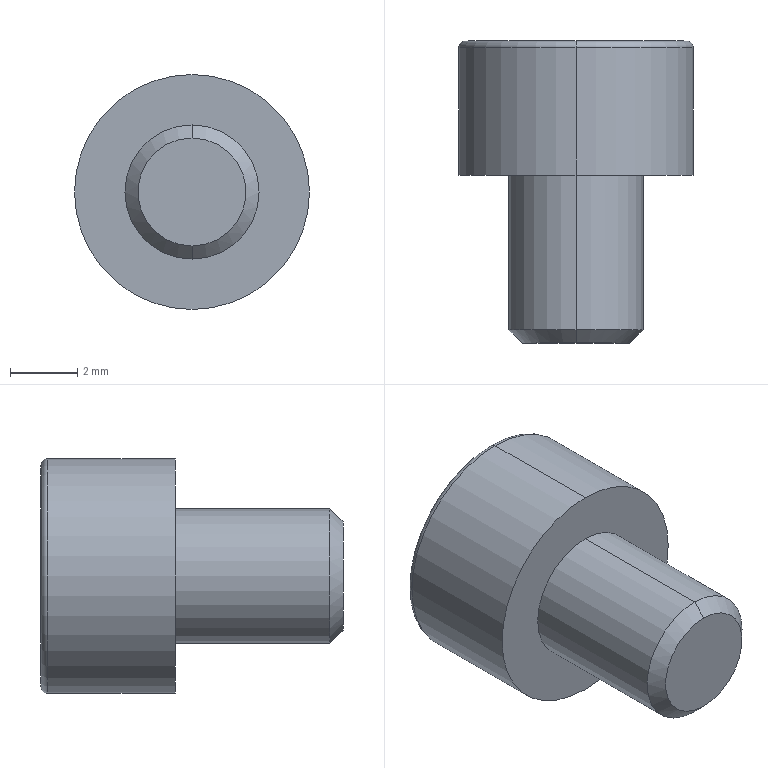Part | STEP file | hex socket M4x0 | 1 solid | 20 faces | box 7 x 9 x 7 mm | volume 199.204 mm3 | plane 10 | cone 4 | cylinder 4 | torus 2 | commonest cylinder face diameters 4 x2 7 x2